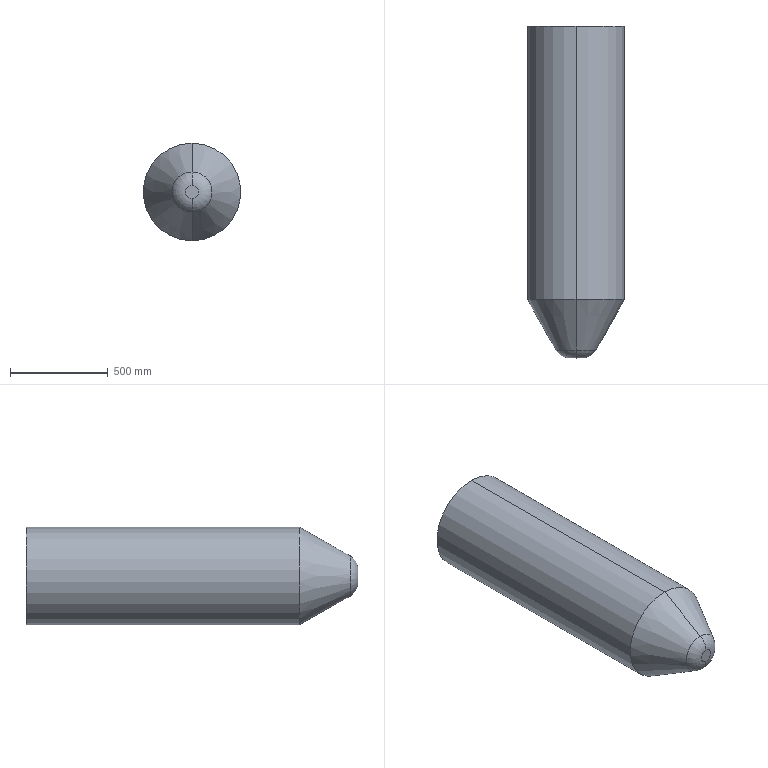Part | SolidWorks | features Fillet 1, Revolution 1, Shell 1 | 1 solid | 15 faces | box 500 x 1700 x 500 mm | volume 151362883 mm3 | torus 4 | cylinder 4 | cone 4 | plane 3 | commonest cylinder face diameters 360 x2 500 x2
STEP:
#1=CARTESIAN_POINT('',(0.,75.07,-42.082));
#2=VERTEX_POINT('',#1);
#3=CARTESIAN_POINT('',(0.,75.07,42.082));
#4=VERTEX_POINT('',#3);
#5=CARTESIAN_POINT('',(0.,75.07,0.));
#6=DIRECTION('',(0.,1.,0.));
#7=DIRECTION('',(0.,0.,1.));
#8=AXIS2_PLACEMENT_3D('',#5,#6,#7);
#9=CIRCLE('',#8,42.082);
#10=EDGE_CURVE('',#2,#4,#9,.T.);
#11=ORIENTED_EDGE('',*,*,#10,.T.);
#12=CARTESIAN_POINT('',(0.,70.,33.382));
#13=VERTEX_POINT('',#12);
#14=CARTESIAN_POINT('',(0.,80.,33.382));
#15=DIRECTION('',(1.,0.,0.));
#16=DIRECTION('',(0.,0.,-1.));
#17=AXIS2_PLACEMENT_3D('',#14,#15,#16);
#18=CIRCLE('',#17,10.);
#19=EDGE_CURVE('',#4,#13,#18,.T.);
#20=ORIENTED_EDGE('',*,*,#19,.T.);
#21=CARTESIAN_POINT('',(0.,70.,-33.382));
#22=VERTEX_POINT('',#21);
#23=CARTESIAN_POINT('',(0.,70.,0.));
#24=DIRECTION('',(0.,-1.,0.));
#25=DIRECTION('',(0.,0.,-1.));
#26=AXIS2_PLACEMENT_3D('',#23,#24,#25);
#27=CIRCLE('',#26,33.382);
#28=EDGE_CURVE('',#13,#22,#27,.T.);
#29=ORIENTED_EDGE('',*,*,#28,.T.);
#30=CARTESIAN_POINT('',(0.,80.,-33.382));
#31=DIRECTION('',(-1.,0.,0.));
#32=DIRECTION('',(0.,0.,1.));
#33=AXIS2_PLACEMENT_3D('',#30,#31,#32);
#34=CIRCLE('',#33,10.);
#35=EDGE_CURVE('',#2,#22,#34,.T.);
#36=ORIENTED_EDGE('',*,*,#35,.F.);
#37=EDGE_LOOP('',(#11,#20,#29,#36));
#38=FACE_OUTER_BOUND('',#37,.T.);
#39=CARTESIAN_POINT('',(0.,80.,0.));
#40=DIRECTION('',(0.,-1.,0.));
#41=DIRECTION('',(0.,0.,-1.));
#42=AXIS2_PLACEMENT_3D('',#39,#40,#41);
#43=TOROIDAL_SURFACE('',#42,33.382,10.);
#44=ADVANCED_FACE('',(#38),#43,.F.);
#45=CARTESIAN_POINT('',(0.,1700.,180.));
#46=VERTEX_POINT('',#45);
#47=CARTESIAN_POINT('',(0.,1700.,-180.));
#48=VERTEX_POINT('',#47);
#49=CARTESIAN_POINT('',(0.,1700.,0.));
#50=DIRECTION('',(0.,-1.,0.));
#51=DIRECTION('',(0.,0.,1.));
#52=AXIS2_PLACEMENT_3D('',#49,#50,#51);
#53=CIRCLE('',#52,180.);
#54=EDGE_CURVE('',#46,#48,#53,.T.);
#55=ORIENTED_EDGE('',*,*,#54,.F.);
#56=CARTESIAN_POINT('',(0.,318.455,180.));
#57=VERTEX_POINT('',#56);
#58=CARTESIAN_POINT('',(0.,0.,180.));
#59=DIRECTION('',(0.,-1.,0.));
#60=VECTOR('',#59,1000.);
#61=LINE('',#58,#60);
#62=EDGE_CURVE('',#46,#57,#61,.T.);
#63=ORIENTED_EDGE('',*,*,#62,.T.);
#64=CARTESIAN_POINT('',(0.,318.455,-180.));
#65=VERTEX_POINT('',#64);
#66=CARTESIAN_POINT('',(0.,318.455,0.));
#67=DIRECTION('',(0.,-1.,0.));
#68=DIRECTION('',(0.,0.,1.));
#69=AXIS2_PLACEMENT_3D('',#66,#67,#68);
#70=CIRCLE('',#69,180.);
#71=EDGE_CURVE('',#57,#65,#70,.T.);
#72=ORIENTED_EDGE('',*,*,#71,.T.);
#73=CARTESIAN_POINT('',(0.,0.,-180.));
#74=DIRECTION('',(0.,-1.,0.));
#75=VECTOR('',#74,1000.);
#76=LINE('',#73,#75);
#77=EDGE_CURVE('',#48,#65,#76,.T.);
#78=ORIENTED_EDGE('',*,*,#77,.F.);
#79=EDGE_LOOP('',(#55,#63,#72,#78));
#80=FACE_OUTER_BOUND('',#79,.T.);
#81=CARTESIAN_POINT('',(0.,0.,0.));
#82=DIRECTION('',(0.,-1.,0.));
#83=DIRECTION('',(0.,0.,-1.));
#84=AXIS2_PLACEMENT_3D('',#81,#82,#83);
#85=CYLINDRICAL_SURFACE('',#84,180.);
#86=ADVANCED_FACE('',(#80),#85,.F.);
#87=ORIENTED_EDGE('',*,*,#10,.F.);
#88=CARTESIAN_POINT('',(0.,34.511,-19.098));
#89=DIRECTION('',(0.,0.87,-0.493));
#90=VECTOR('',#89,1000.);
#91=LINE('',#88,#90);
#92=EDGE_CURVE('',#2,#65,#91,.T.);
#93=ORIENTED_EDGE('',*,*,#92,.T.);
#94=ORIENTED_EDGE('',*,*,#71,.F.);
#95=CARTESIAN_POINT('',(0.,34.511,19.098));
#96=DIRECTION('',(0.,0.87,0.493));
#97=VECTOR('',#96,1000.);
#98=LINE('',#95,#97);
#99=EDGE_CURVE('',#4,#57,#98,.T.);
#100=ORIENTED_EDGE('',*,*,#99,.F.);
#101=EDGE_LOOP('',(#87,#93,#94,#100));
#102=FACE_OUTER_BOUND('',#101,.T.);
#103=CARTESIAN_POINT('',(0.,34.511,0.));
#104=DIRECTION('',(0.,1.,0.));
#105=DIRECTION('',(0.,0.,1.));
#106=AXIS2_PLACEMENT_3D('',#103,#104,#105);
#107=CONICAL_SURFACE('',#106,19.098,0.5155);
#108=ADVANCED_FACE('',(#102),#107,.F.);
#109=CARTESIAN_POINT('',(0.,40.559,102.983));
#110=VERTEX_POINT('',#109);
#111=CARTESIAN_POINT('',(0.,40.559,-102.983));
#112=VERTEX_POINT('',#111);
#113=CARTESIAN_POINT('',(0.,40.559,0.));
#114=DIRECTION('',(0.,1.,0.));
#115=DIRECTION('',(0.,0.,-1.));
#116=AXIS2_PLACEMENT_3D('',#113,#114,#115);
#117=CIRCLE('',#116,102.983);
#118=EDGE_CURVE('',#110,#112,#117,.T.);
#119=ORIENTED_EDGE('',*,*,#118,.F.);
#120=CARTESIAN_POINT('',(0.,0.,33.382));
#121=VERTEX_POINT('',#120);
#122=CARTESIAN_POINT('',(0.,80.,33.382));
#123=DIRECTION('',(1.,0.,0.));
#124=DIRECTION('',(0.,0.,-1.));
#125=AXIS2_PLACEMENT_3D('',#122,#123,#124);
#126=CIRCLE('',#125,80.);
#127=EDGE_CURVE('',#110,#121,#126,.T.);
#128=ORIENTED_EDGE('',*,*,#127,.T.);
#129=CARTESIAN_POINT('',(0.,0.,-33.382));
#130=VERTEX_POINT('',#129);
#131=CARTESIAN_POINT('',(0.,0.,0.));
#132=DIRECTION('',(0.,-1.,0.));
#133=DIRECTION('',(0.,0.,-1.));
#134=AXIS2_PLACEMENT_3D('',#131,#132,#133);
#135=CIRCLE('',#134,33.382);
#136=EDGE_CURVE('',#130,#121,#135,.T.);
#137=ORIENTED_EDGE('',*,*,#136,.F.);
#138=CARTESIAN_POINT('',(0.,80.,-33.382));
#139=DIRECTION('',(-1.,0.,0.));
#140=DIRECTION('',(0.,0.,1.));
#141=AXIS2_PLACEMENT_3D('',#138,#139,#140);
#142=CIRCLE('',#141,80.);
#143=EDGE_CURVE('',#112,#130,#142,.T.);
#144=ORIENTED_EDGE('',*,*,#143,.F.);
#145=EDGE_LOOP('',(#119,#128,#137,#144));
#146=FACE_OUTER_BOUND('',#145,.T.);
#147=CARTESIAN_POINT('',(0.,80.,0.));
#148=DIRECTION('',(0.,-1.,0.));
#149=DIRECTION('',(0.,0.,-1.));
#150=AXIS2_PLACEMENT_3D('',#147,#148,#149);
#151=TOROIDAL_SURFACE('',#150,33.382,80.);
#152=ADVANCED_FACE('',(#146),#151,.T.);
#153=CARTESIAN_POINT('',(0.,1700.,-250.));
#154=VERTEX_POINT('',#153);
#155=CARTESIAN_POINT('',(0.,1700.,250.));
#156=VERTEX_POINT('',#155);
#157=CARTESIAN_POINT('',(0.,1700.,0.));
#158=DIRECTION('',(0.,-1.,0.));
#159=DIRECTION('',(0.,0.,-1.));
#160=AXIS2_PLACEMENT_3D('',#157,#158,#159);
#161=CIRCLE('',#160,250.);
#162=EDGE_CURVE('',#154,#156,#161,.T.);
#163=ORIENTED_EDGE('',*,*,#162,.T.);
#164=CARTESIAN_POINT('',(0.,300.,250.));
#165=VERTEX_POINT('',#164);
#166=CARTESIAN_POINT('',(0.,0.,250.));
#167=DIRECTION('',(0.,-1.,0.));
#168=VECTOR('',#167,1000.);
#169=LINE('',#166,#168);
#170=EDGE_CURVE('',#156,#165,#169,.T.);
#171=ORIENTED_EDGE('',*,*,#170,.T.);
#172=CARTESIAN_POINT('',(0.,300.,-250.));
#173=VERTEX_POINT('',#172);
#174=CARTESIAN_POINT('',(0.,300.,0.));
#175=DIRECTION('',(0.,-1.,0.));
#176=DIRECTION('',(0.,0.,-1.));
#177=AXIS2_PLACEMENT_3D('',#174,#175,#176);
#178=CIRCLE('',#177,250.);
#179=EDGE_CURVE('',#173,#165,#178,.T.);
#180=ORIENTED_EDGE('',*,*,#179,.F.);
#181=CARTESIAN_POINT('',(0.,0.,-250.));
#182=DIRECTION('',(0.,-1.,0.));
#183=VECTOR('',#182,1000.);
#184=LINE('',#181,#183);
#185=EDGE_CURVE('',#154,#173,#184,.T.);
#186=ORIENTED_EDGE('',*,*,#185,.F.);
#187=EDGE_LOOP('',(#163,#171,#180,#186));
#188=FACE_OUTER_BOUND('',#187,.T.);
#189=CARTESIAN_POINT('',(0.,0.,0.));
#190=DIRECTION('',(0.,-1.,0.));
#191=DIRECTION('',(0.,0.,-1.));
#192=AXIS2_PLACEMENT_3D('',#189,#190,#191);
#193=CYLINDRICAL_SURFACE('',#192,250.);
#194=ADVANCED_FACE('',(#188),#193,.T.);
#195=ORIENTED_EDGE('',*,*,#118,.T.);
#196=CARTESIAN_POINT('',(0.,0.,-80.));
#197=DIRECTION('',(0.,0.87,-0.493));
#198=VECTOR('',#197,1000.);
#199=LINE('',#196,#198);
#200=EDGE_CURVE('',#112,#173,#199,.T.);
#201=ORIENTED_EDGE('',*,*,#200,.T.);
#202=ORIENTED_EDGE('',*,*,#179,.T.);
#203=CARTESIAN_POINT('',(0.,0.,80.));
#204=DIRECTION('',(0.,0.87,0.493));
#205=VECTOR('',#204,1000.);
#206=LINE('',#203,#205);
#207=EDGE_CURVE('',#110,#165,#206,.T.);
#208=ORIENTED_EDGE('',*,*,#207,.F.);
#209=EDGE_LOOP('',(#195,#201,#202,#208));
#210=FACE_OUTER_BOUND('',#209,.T.);
#211=CARTESIAN_POINT('',(0.,0.,0.));
#212=DIRECTION('',(0.,1.,0.));
#213=DIRECTION('',(0.,0.,1.));
#214=AXIS2_PLACEMENT_3D('',#211,#212,#213);
#215=CONICAL_SURFACE('',#214,80.,0.5155);
#216=ADVANCED_FACE('',(#210),#215,.T.);
#217=ORIENTED_EDGE('',*,*,#136,.T.);
#218=CARTESIAN_POINT('',(0.,0.,0.));
#219=DIRECTION('',(0.,-1.,0.));
#220=DIRECTION('',(0.,0.,-1.));
#221=AXIS2_PLACEMENT_3D('',#218,#219,#220);
#222=CIRCLE('',#221,33.382);
#223=EDGE_CURVE('',#121,#130,#222,.T.);
#224=ORIENTED_EDGE('',*,*,#223,.T.);
#225=EDGE_LOOP('',(#217,#224));
#226=FACE_OUTER_BOUND('',#225,.T.);
#227=CARTESIAN_POINT('',(0.,0.,0.));
#228=DIRECTION('',(0.,-1.,0.));
#229=DIRECTION('',(0.,0.,-1.));
#230=AXIS2_PLACEMENT_3D('',#227,#228,#229);
#231=PLANE('',#230);
#232=ADVANCED_FACE('',(#226),#231,.T.);
#233=ORIENTED_EDGE('',*,*,#200,.F.);
#234=CARTESIAN_POINT('',(0.,40.559,0.));
#235=DIRECTION('',(0.,1.,0.));
#236=DIRECTION('',(0.,0.,-1.));
#237=AXIS2_PLACEMENT_3D('',#234,#235,#236);
#238=CIRCLE('',#237,102.983);
#239=EDGE_CURVE('',#112,#110,#238,.T.);
#240=ORIENTED_EDGE('',*,*,#239,.T.);
#241=ORIENTED_EDGE('',*,*,#207,.T.);
#242=CARTESIAN_POINT('',(0.,300.,0.));
#243=DIRECTION('',(0.,-1.,0.));
#244=DIRECTION('',(0.,0.,-1.));
#245=AXIS2_PLACEMENT_3D('',#242,#243,#244);
#246=CIRCLE('',#245,250.);
#247=EDGE_CURVE('',#165,#173,#246,.T.);
#248=ORIENTED_EDGE('',*,*,#247,.T.);
#249=EDGE_LOOP('',(#233,#240,#241,#248));
#250=FACE_OUTER_BOUND('',#249,.T.);
#251=CARTESIAN_POINT('',(0.,0.,0.));
#252=DIRECTION('',(0.,1.,0.));
#253=DIRECTION('',(0.,0.,1.));
#254=AXIS2_PLACEMENT_3D('',#251,#252,#253);
#255=CONICAL_SURFACE('',#254,80.,0.5155);
#256=ADVANCED_FACE('',(#250),#255,.T.);
#257=ORIENTED_EDGE('',*,*,#170,.F.);
#258=CARTESIAN_POINT('',(0.,1700.,0.));
#259=DIRECTION('',(0.,-1.,0.));
#260=DIRECTION('',(0.,0.,-1.));
#261=AXIS2_PLACEMENT_3D('',#258,#259,#260);
#262=CIRCLE('',#261,250.);
#263=EDGE_CURVE('',#156,#154,#262,.T.);
#264=ORIENTED_EDGE('',*,*,#263,.T.);
#265=ORIENTED_EDGE('',*,*,#185,.T.);
#266=ORIENTED_EDGE('',*,*,#247,.F.);
#267=EDGE_LOOP('',(#257,#264,#265,#266));
#268=FACE_OUTER_BOUND('',#267,.T.);
#269=CARTESIAN_POINT('',(0.,0.,0.));
#270=DIRECTION('',(0.,-1.,0.));
#271=DIRECTION('',(0.,0.,-1.));
#272=AXIS2_PLACEMENT_3D('',#269,#270,#271);
#273=CYLINDRICAL_SURFACE('',#272,250.);
#274=ADVANCED_FACE('',(#268),#273,.T.);
#275=CARTESIAN_POINT('',(0.,1700.,0.));
#276=DIRECTION('',(0.,-1.,0.));
#277=DIRECTION('',(0.,0.,1.));
#278=AXIS2_PLACEMENT_3D('',#275,#276,#277);
#279=CIRCLE('',#278,180.);
#280=EDGE_CURVE('',#48,#46,#279,.T.);
#281=ORIENTED_EDGE('',*,*,#280,.T.);
#282=ORIENTED_EDGE('',*,*,#54,.T.);
#283=EDGE_LOOP('',(#281,#282));
#284=FACE_BOUND('',#283,.T.);
#285=ORIENTED_EDGE('',*,*,#162,.F.);
#286=ORIENTED_EDGE('',*,*,#263,.F.);
#287=EDGE_LOOP('',(#285,#286));
#288=FACE_OUTER_BOUND('',#287,.T.);
#289=CARTESIAN_POINT('',(0.,1700.,0.));
#290=DIRECTION('',(0.,1.,0.));
#291=DIRECTION('',(0.,0.,1.));
#292=AXIS2_PLACEMENT_3D('',#289,#290,#291);
#293=PLANE('',#292);
#294=ADVANCED_FACE('',(#284,#288),#293,.T.);
#295=ORIENTED_EDGE('',*,*,#127,.F.);
#296=ORIENTED_EDGE('',*,*,#239,.F.);
#297=ORIENTED_EDGE('',*,*,#143,.T.);
#298=ORIENTED_EDGE('',*,*,#223,.F.);
#299=EDGE_LOOP('',(#295,#296,#297,#298));
#300=FACE_OUTER_BOUND('',#299,.T.);
#301=CARTESIAN_POINT('',(0.,80.,0.));
#302=DIRECTION('',(0.,-1.,0.));
#303=DIRECTION('',(0.,0.,-1.));
#304=AXIS2_PLACEMENT_3D('',#301,#302,#303);
#305=TOROIDAL_SURFACE('',#304,33.382,80.);
#306=ADVANCED_FACE('',(#300),#305,.T.);
#307=CARTESIAN_POINT('',(0.,70.,0.));
#308=DIRECTION('',(0.,-1.,0.));
#309=DIRECTION('',(0.,0.,-1.));
#310=AXIS2_PLACEMENT_3D('',#307,#308,#309);
#311=CIRCLE('',#310,33.382);
#312=EDGE_CURVE('',#22,#13,#311,.T.);
#313=ORIENTED_EDGE('',*,*,#312,.F.);
#314=ORIENTED_EDGE('',*,*,#28,.F.);
#315=EDGE_LOOP('',(#313,#314));
#316=FACE_OUTER_BOUND('',#315,.T.);
#317=CARTESIAN_POINT('',(0.,70.,0.));
#318=DIRECTION('',(0.,-1.,0.));
#319=DIRECTION('',(0.,0.,-1.));
#320=AXIS2_PLACEMENT_3D('',#317,#318,#319);
#321=PLANE('',#320);
#322=ADVANCED_FACE('',(#316),#321,.F.);
#323=ORIENTED_EDGE('',*,*,#92,.F.);
#324=CARTESIAN_POINT('',(0.,75.07,0.));
#325=DIRECTION('',(0.,1.,0.));
#326=DIRECTION('',(0.,0.,1.));
#327=AXIS2_PLACEMENT_3D('',#324,#325,#326);
#328=CIRCLE('',#327,42.082);
#329=EDGE_CURVE('',#4,#2,#328,.T.);
#330=ORIENTED_EDGE('',*,*,#329,.F.);
#331=ORIENTED_EDGE('',*,*,#99,.T.);
#332=CARTESIAN_POINT('',(0.,318.455,0.));
#333=DIRECTION('',(0.,-1.,0.));
#334=DIRECTION('',(0.,0.,1.));
#335=AXIS2_PLACEMENT_3D('',#332,#333,#334);
#336=CIRCLE('',#335,180.);
#337=EDGE_CURVE('',#65,#57,#336,.T.);
#338=ORIENTED_EDGE('',*,*,#337,.F.);
#339=EDGE_LOOP('',(#323,#330,#331,#338));
#340=FACE_OUTER_BOUND('',#339,.T.);
#341=CARTESIAN_POINT('',(0.,34.511,0.));
#342=DIRECTION('',(0.,1.,0.));
#343=DIRECTION('',(0.,0.,1.));
#344=AXIS2_PLACEMENT_3D('',#341,#342,#343);
#345=CONICAL_SURFACE('',#344,19.098,0.5155);
#346=ADVANCED_FACE('',(#340),#345,.F.);
#347=ORIENTED_EDGE('',*,*,#62,.F.);
#348=ORIENTED_EDGE('',*,*,#280,.F.);
#349=ORIENTED_EDGE('',*,*,#77,.T.);
#350=ORIENTED_EDGE('',*,*,#337,.T.);
#351=EDGE_LOOP('',(#347,#348,#349,#350));
#352=FACE_OUTER_BOUND('',#351,.T.);
#353=CARTESIAN_POINT('',(0.,0.,0.));
#354=DIRECTION('',(0.,-1.,0.));
#355=DIRECTION('',(0.,0.,-1.));
#356=AXIS2_PLACEMENT_3D('',#353,#354,#355);
#357=CYLINDRICAL_SURFACE('',#356,180.);
#358=ADVANCED_FACE('',(#352),#357,.F.);
#359=ORIENTED_EDGE('',*,*,#19,.F.);
#360=ORIENTED_EDGE('',*,*,#329,.T.);
#361=ORIENTED_EDGE('',*,*,#35,.T.);
#362=ORIENTED_EDGE('',*,*,#312,.T.);
#363=EDGE_LOOP('',(#359,#360,#361,#362));
#364=FACE_OUTER_BOUND('',#363,.T.);
#365=CARTESIAN_POINT('',(0.,80.,0.));
#366=DIRECTION('',(0.,-1.,0.));
#367=DIRECTION('',(0.,0.,-1.));
#368=AXIS2_PLACEMENT_3D('',#365,#366,#367);
#369=TOROIDAL_SURFACE('',#368,33.382,10.);
#370=ADVANCED_FACE('',(#364),#369,.F.);
#371=CLOSED_SHELL('',(#44,#86,#108,#152,#194,#216,#232,#256,#274,#294,#306,#322,#346,#358,#370));
#372=MANIFOLD_SOLID_BREP('',#371);
#373=CARTESIAN_POINT('',(0.,0.,0.));
#374=DIRECTION('',(0.,0.,1.));
#375=DIRECTION('',(1.,0.,0.));
#376=AXIS2_PLACEMENT_3D('',#373,#374,#375);
#377=(LENGTH_UNIT()NAMED_UNIT(*)SI_UNIT(.MILLI.,.METRE.));
#378=UNCERTAINTY_MEASURE_WITH_UNIT(LENGTH_MEASURE(0.00001),#377,'','');
#379=(NAMED_UNIT(*)PLANE_ANGLE_UNIT()SI_UNIT($,.RADIAN.));
#380=(NAMED_UNIT(*)SI_UNIT($,.STERADIAN.)SOLID_ANGLE_UNIT());
#381=(GEOMETRIC_REPRESENTATION_CONTEXT(3)GLOBAL_UNCERTAINTY_ASSIGNED_CONTEXT((#378))GLOBAL_UNIT_ASSIGNED_CONTEXT((#377,#379,#380))REPRESENTATION_CONTEXT('',''));
#382=ADVANCED_BREP_SHAPE_REPRESENTATION('',(#372,#376),#381);